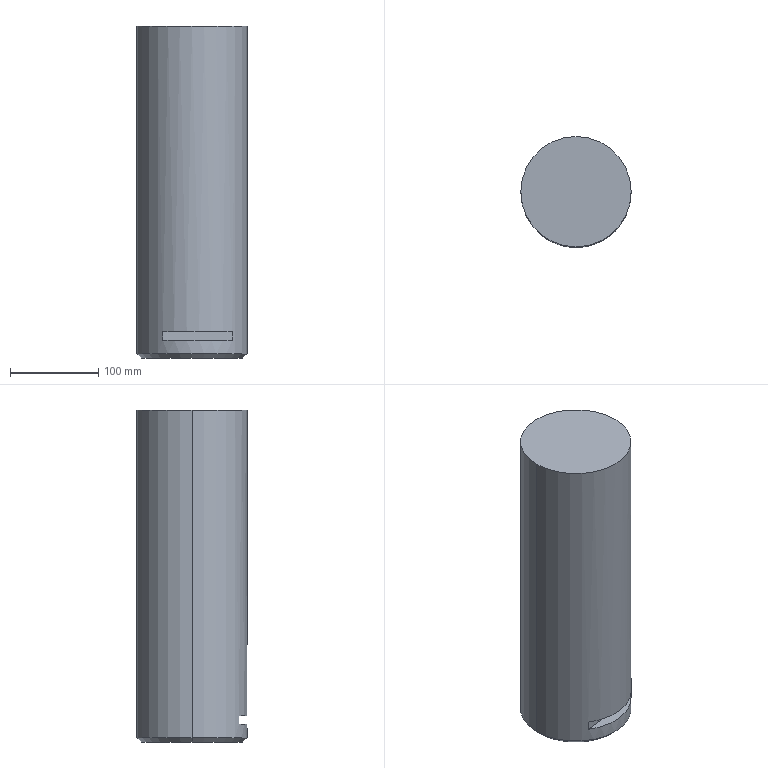Part | SolidWorks | features MirrorStock 1 | 1 solid | 9 faces | box 125 x 125 x 375.881 mm | volume 4600278 mm3 | plane 5 | cone 2 | cylinder 2 | commonest cylinder face diameters 125 x2
STEP:
#1=CARTESIAN_POINT('',(5031.911,2238.406,-30.));
#2=VERTEX_POINT('',#1);
#3=CARTESIAN_POINT('',(5146.911,2238.406,-30.));
#4=VERTEX_POINT('',#3);
#5=CARTESIAN_POINT('',(5089.411,2238.406,-30.));
#6=DIRECTION('',(0.,0.,1.));
#7=DIRECTION('',(1.,0.,0.));
#8=AXIS2_PLACEMENT_3D('',#5,#6,#7);
#9=CIRCLE('',#8,57.5);
#10=EDGE_CURVE('',#2,#4,#9,.T.);
#11=ORIENTED_EDGE('',*,*,#10,.T.);
#12=CARTESIAN_POINT('',(5151.911,2238.406,-25.));
#13=VERTEX_POINT('',#12);
#14=CARTESIAN_POINT('',(5146.911,2238.406,-30.));
#15=DIRECTION('',(0.7071,0.,0.7071));
#16=VECTOR('',#15,1000.);
#17=LINE('',#14,#16);
#18=EDGE_CURVE('',#4,#13,#17,.T.);
#19=ORIENTED_EDGE('',*,*,#18,.T.);
#20=CARTESIAN_POINT('',(5026.911,2238.406,-25.));
#21=VERTEX_POINT('',#20);
#22=CARTESIAN_POINT('',(5089.411,2238.406,-25.));
#23=DIRECTION('',(0.,0.,-1.));
#24=DIRECTION('',(1.,0.,0.));
#25=AXIS2_PLACEMENT_3D('',#22,#23,#24);
#26=CIRCLE('',#25,62.5);
#27=EDGE_CURVE('',#13,#21,#26,.T.);
#28=ORIENTED_EDGE('',*,*,#27,.T.);
#29=CARTESIAN_POINT('',(5031.911,2238.406,-30.));
#30=DIRECTION('',(-0.7071,0.,0.7071));
#31=VECTOR('',#30,1000.);
#32=LINE('',#29,#31);
#33=EDGE_CURVE('',#2,#21,#32,.T.);
#34=ORIENTED_EDGE('',*,*,#33,.F.);
#35=EDGE_LOOP('',(#11,#19,#28,#34));
#36=FACE_OUTER_BOUND('',#35,.T.);
#37=CARTESIAN_POINT('',(5089.411,2238.406,-30.));
#38=DIRECTION('',(0.,0.,1.));
#39=DIRECTION('',(-1.,0.,0.));
#40=AXIS2_PLACEMENT_3D('',#37,#38,#39);
#41=CONICAL_SURFACE('',#40,57.5,0.7854);
#42=ADVANCED_FACE('',(#36),#41,.T.);
#43=CARTESIAN_POINT('',(5056.406,2185.331,0.));
#44=VERTEX_POINT('',#43);
#45=CARTESIAN_POINT('',(5135.037,2195.692,0.));
#46=VERTEX_POINT('',#45);
#47=CARTESIAN_POINT('',(5089.411,2238.406,0.));
#48=DIRECTION('',(0.,0.,1.));
#49=DIRECTION('',(1.,0.,0.));
#50=AXIS2_PLACEMENT_3D('',#47,#48,#49);
#51=CIRCLE('',#50,62.5);
#52=EDGE_CURVE('',#44,#46,#51,.T.);
#53=ORIENTED_EDGE('',*,*,#52,.T.);
#54=CARTESIAN_POINT('',(5135.037,2195.692,-10.));
#55=VERTEX_POINT('',#54);
#56=CARTESIAN_POINT('',(5135.037,2195.692,-10.));
#57=DIRECTION('',(0.,0.,1.));
#58=VECTOR('',#57,1000.);
#59=LINE('',#56,#58);
#60=EDGE_CURVE('',#55,#46,#59,.T.);
#61=ORIENTED_EDGE('',*,*,#60,.F.);
#62=CARTESIAN_POINT('',(5056.406,2185.331,-10.));
#63=VERTEX_POINT('',#62);
#64=CARTESIAN_POINT('',(5089.411,2238.406,-10.));
#65=DIRECTION('',(0.,0.,1.));
#66=DIRECTION('',(1.,0.,0.));
#67=AXIS2_PLACEMENT_3D('',#64,#65,#66);
#68=CIRCLE('',#67,62.5);
#69=EDGE_CURVE('',#63,#55,#68,.T.);
#70=ORIENTED_EDGE('',*,*,#69,.F.);
#71=CARTESIAN_POINT('',(5056.406,2185.331,-10.));
#72=DIRECTION('',(0.,0.,1.));
#73=VECTOR('',#72,1000.);
#74=LINE('',#71,#73);
#75=EDGE_CURVE('',#63,#44,#74,.T.);
#76=ORIENTED_EDGE('',*,*,#75,.T.);
#77=EDGE_LOOP('',(#53,#61,#70,#76));
#78=FACE_BOUND('',#77,.T.);
#79=CARTESIAN_POINT('',(5151.911,2238.406,345.881));
#80=VERTEX_POINT('',#79);
#81=CARTESIAN_POINT('',(5026.911,2238.406,345.881));
#82=VERTEX_POINT('',#81);
#83=CARTESIAN_POINT('',(5089.411,2238.406,345.881));
#84=DIRECTION('',(0.,0.,-1.));
#85=DIRECTION('',(1.,0.,0.));
#86=AXIS2_PLACEMENT_3D('',#83,#84,#85);
#87=CIRCLE('',#86,62.5);
#88=EDGE_CURVE('',#80,#82,#87,.T.);
#89=ORIENTED_EDGE('',*,*,#88,.T.);
#90=CARTESIAN_POINT('',(5026.911,2238.406,522.657));
#91=DIRECTION('',(0.,0.,-1.));
#92=VECTOR('',#91,1000.);
#93=LINE('',#90,#92);
#94=EDGE_CURVE('',#82,#21,#93,.T.);
#95=ORIENTED_EDGE('',*,*,#94,.T.);
#96=ORIENTED_EDGE('',*,*,#27,.F.);
#97=CARTESIAN_POINT('',(5151.911,2238.406,522.657));
#98=DIRECTION('',(0.,0.,-1.));
#99=VECTOR('',#98,1000.);
#100=LINE('',#97,#99);
#101=EDGE_CURVE('',#80,#13,#100,.T.);
#102=ORIENTED_EDGE('',*,*,#101,.F.);
#103=EDGE_LOOP('',(#89,#95,#96,#102));
#104=FACE_OUTER_BOUND('',#103,.T.);
#105=CARTESIAN_POINT('',(5089.411,2238.406,522.657));
#106=DIRECTION('',(0.,0.,-1.));
#107=DIRECTION('',(1.,0.,0.));
#108=AXIS2_PLACEMENT_3D('',#105,#106,#107);
#109=CYLINDRICAL_SURFACE('',#108,62.5);
#110=ADVANCED_FACE('',(#78,#104),#109,.T.);
#111=ORIENTED_EDGE('',*,*,#52,.F.);
#112=CARTESIAN_POINT('',(-196.746,1493.143,0.));
#113=DIRECTION('',(-0.9914,-0.1306,0.));
#114=VECTOR('',#113,1000.);
#115=LINE('',#112,#114);
#116=EDGE_CURVE('',#46,#44,#115,.T.);
#117=ORIENTED_EDGE('',*,*,#116,.F.);
#118=EDGE_LOOP('',(#111,#117));
#119=FACE_OUTER_BOUND('',#118,.T.);
#120=CARTESIAN_POINT('',(5089.411,2238.406,0.));
#121=DIRECTION('',(0.,0.,-1.));
#122=DIRECTION('',(1.,0.,0.));
#123=AXIS2_PLACEMENT_3D('',#120,#121,#122);
#124=PLANE('',#123);
#125=ADVANCED_FACE('',(#119),#124,.T.);
#126=ORIENTED_EDGE('',*,*,#94,.F.);
#127=CARTESIAN_POINT('',(5089.411,2238.406,345.881));
#128=DIRECTION('',(0.,0.,-1.));
#129=DIRECTION('',(1.,0.,0.));
#130=AXIS2_PLACEMENT_3D('',#127,#128,#129);
#131=CIRCLE('',#130,62.5);
#132=EDGE_CURVE('',#82,#80,#131,.T.);
#133=ORIENTED_EDGE('',*,*,#132,.T.);
#134=ORIENTED_EDGE('',*,*,#101,.T.);
#135=CARTESIAN_POINT('',(5089.411,2238.406,-25.));
#136=DIRECTION('',(0.,0.,-1.));
#137=DIRECTION('',(1.,0.,0.));
#138=AXIS2_PLACEMENT_3D('',#135,#136,#137);
#139=CIRCLE('',#138,62.5);
#140=EDGE_CURVE('',#21,#13,#139,.T.);
#141=ORIENTED_EDGE('',*,*,#140,.F.);
#142=EDGE_LOOP('',(#126,#133,#134,#141));
#143=FACE_OUTER_BOUND('',#142,.T.);
#144=CARTESIAN_POINT('',(5089.411,2238.406,522.657));
#145=DIRECTION('',(0.,0.,-1.));
#146=DIRECTION('',(1.,0.,0.));
#147=AXIS2_PLACEMENT_3D('',#144,#145,#146);
#148=CYLINDRICAL_SURFACE('',#147,62.5);
#149=ADVANCED_FACE('',(#143),#148,.T.);
#150=ORIENTED_EDGE('',*,*,#88,.F.);
#151=ORIENTED_EDGE('',*,*,#132,.F.);
#152=EDGE_LOOP('',(#150,#151));
#153=FACE_OUTER_BOUND('',#152,.T.);
#154=CARTESIAN_POINT('',(5360.292,2632.168,345.881));
#155=DIRECTION('',(0.,0.,-1.));
#156=DIRECTION('',(-0.9914,-0.1306,0.));
#157=AXIS2_PLACEMENT_3D('',#154,#155,#156);
#158=PLANE('',#157);
#159=ADVANCED_FACE('',(#153),#158,.F.);
#160=ORIENTED_EDGE('',*,*,#116,.T.);
#161=ORIENTED_EDGE('',*,*,#75,.F.);
#162=CARTESIAN_POINT('',(-196.746,1493.143,-10.));
#163=DIRECTION('',(-0.9914,-0.1306,0.));
#164=VECTOR('',#163,1000.);
#165=LINE('',#162,#164);
#166=EDGE_CURVE('',#55,#63,#165,.T.);
#167=ORIENTED_EDGE('',*,*,#166,.F.);
#168=ORIENTED_EDGE('',*,*,#60,.T.);
#169=EDGE_LOOP('',(#160,#161,#167,#168));
#170=FACE_OUTER_BOUND('',#169,.T.);
#171=CARTESIAN_POINT('',(-196.746,1493.143,-10.));
#172=DIRECTION('',(0.1306,-0.9914,0.));
#173=DIRECTION('',(0.9914,0.1306,0.));
#174=AXIS2_PLACEMENT_3D('',#171,#172,#173);
#175=PLANE('',#174);
#176=ADVANCED_FACE('',(#170),#175,.T.);
#177=ORIENTED_EDGE('',*,*,#10,.F.);
#178=CARTESIAN_POINT('',(5089.411,2238.406,-30.));
#179=DIRECTION('',(0.,0.,1.));
#180=DIRECTION('',(1.,0.,0.));
#181=AXIS2_PLACEMENT_3D('',#178,#179,#180);
#182=CIRCLE('',#181,57.5);
#183=EDGE_CURVE('',#4,#2,#182,.T.);
#184=ORIENTED_EDGE('',*,*,#183,.F.);
#185=EDGE_LOOP('',(#177,#184));
#186=FACE_OUTER_BOUND('',#185,.T.);
#187=CARTESIAN_POINT('',(5089.411,2238.406,-30.));
#188=DIRECTION('',(0.,0.,-1.));
#189=DIRECTION('',(1.,0.,0.));
#190=AXIS2_PLACEMENT_3D('',#187,#188,#189);
#191=PLANE('',#190);
#192=ADVANCED_FACE('',(#186),#191,.T.);
#193=ORIENTED_EDGE('',*,*,#166,.T.);
#194=ORIENTED_EDGE('',*,*,#69,.T.);
#195=EDGE_LOOP('',(#193,#194));
#196=FACE_OUTER_BOUND('',#195,.T.);
#197=CARTESIAN_POINT('',(5089.411,2238.406,-10.));
#198=DIRECTION('',(0.,0.,-1.));
#199=DIRECTION('',(1.,0.,0.));
#200=AXIS2_PLACEMENT_3D('',#197,#198,#199);
#201=PLANE('',#200);
#202=ADVANCED_FACE('',(#196),#201,.F.);
#203=ORIENTED_EDGE('',*,*,#18,.F.);
#204=ORIENTED_EDGE('',*,*,#183,.T.);
#205=ORIENTED_EDGE('',*,*,#33,.T.);
#206=ORIENTED_EDGE('',*,*,#140,.T.);
#207=EDGE_LOOP('',(#203,#204,#205,#206));
#208=FACE_OUTER_BOUND('',#207,.T.);
#209=CARTESIAN_POINT('',(5089.411,2238.406,-30.));
#210=DIRECTION('',(0.,0.,1.));
#211=DIRECTION('',(-1.,0.,0.));
#212=AXIS2_PLACEMENT_3D('',#209,#210,#211);
#213=CONICAL_SURFACE('',#212,57.5,0.7854);
#214=ADVANCED_FACE('',(#208),#213,.T.);
#215=CLOSED_SHELL('',(#42,#110,#125,#149,#159,#176,#192,#202,#214));
#216=MANIFOLD_SOLID_BREP('',#215);
#217=CARTESIAN_POINT('',(0.,0.,0.));
#218=DIRECTION('',(0.,0.,1.));
#219=DIRECTION('',(1.,0.,0.));
#220=AXIS2_PLACEMENT_3D('',#217,#218,#219);
#221=(LENGTH_UNIT()NAMED_UNIT(*)SI_UNIT(.MILLI.,.METRE.));
#222=UNCERTAINTY_MEASURE_WITH_UNIT(LENGTH_MEASURE(0.00001),#221,'','');
#223=(NAMED_UNIT(*)PLANE_ANGLE_UNIT()SI_UNIT($,.RADIAN.));
#224=(NAMED_UNIT(*)SI_UNIT($,.STERADIAN.)SOLID_ANGLE_UNIT());
#225=(GEOMETRIC_REPRESENTATION_CONTEXT(3)GLOBAL_UNCERTAINTY_ASSIGNED_CONTEXT((#222))GLOBAL_UNIT_ASSIGNED_CONTEXT((#221,#223,#224))REPRESENTATION_CONTEXT('',''));
#226=ADVANCED_BREP_SHAPE_REPRESENTATION('',(#216,#220),#225);